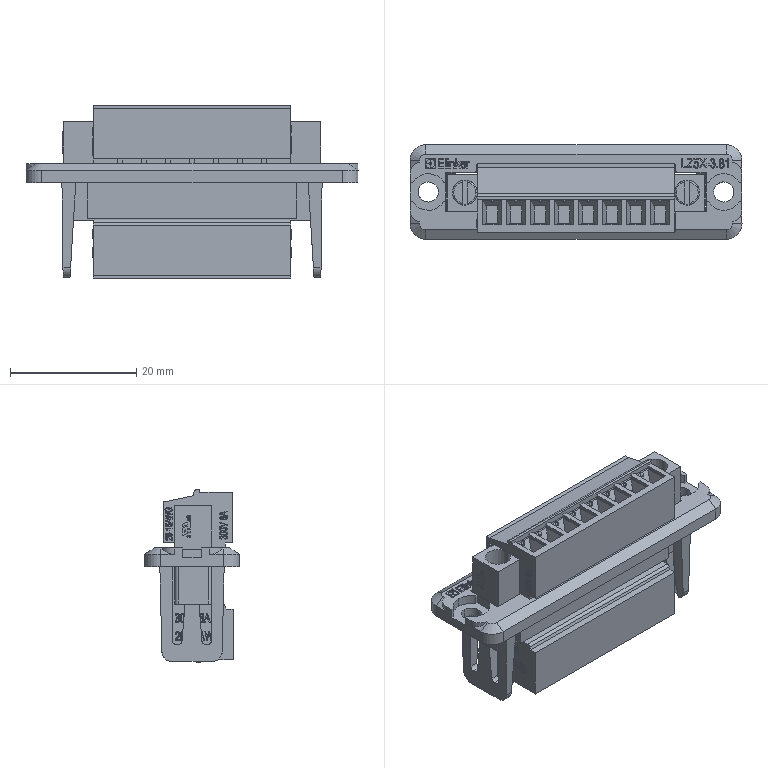Part | NX | features BREP 33 | 33 solids | 5587 faces | volume 9360 mm3 | plane 4486 | spline 471 | cylinder 410 | torus 168 | cone 52 | commonest cylinder face diameters 3.2 x48 3.6 x36 1 x34 2.8 x32 2.94 x32 2.5 x26